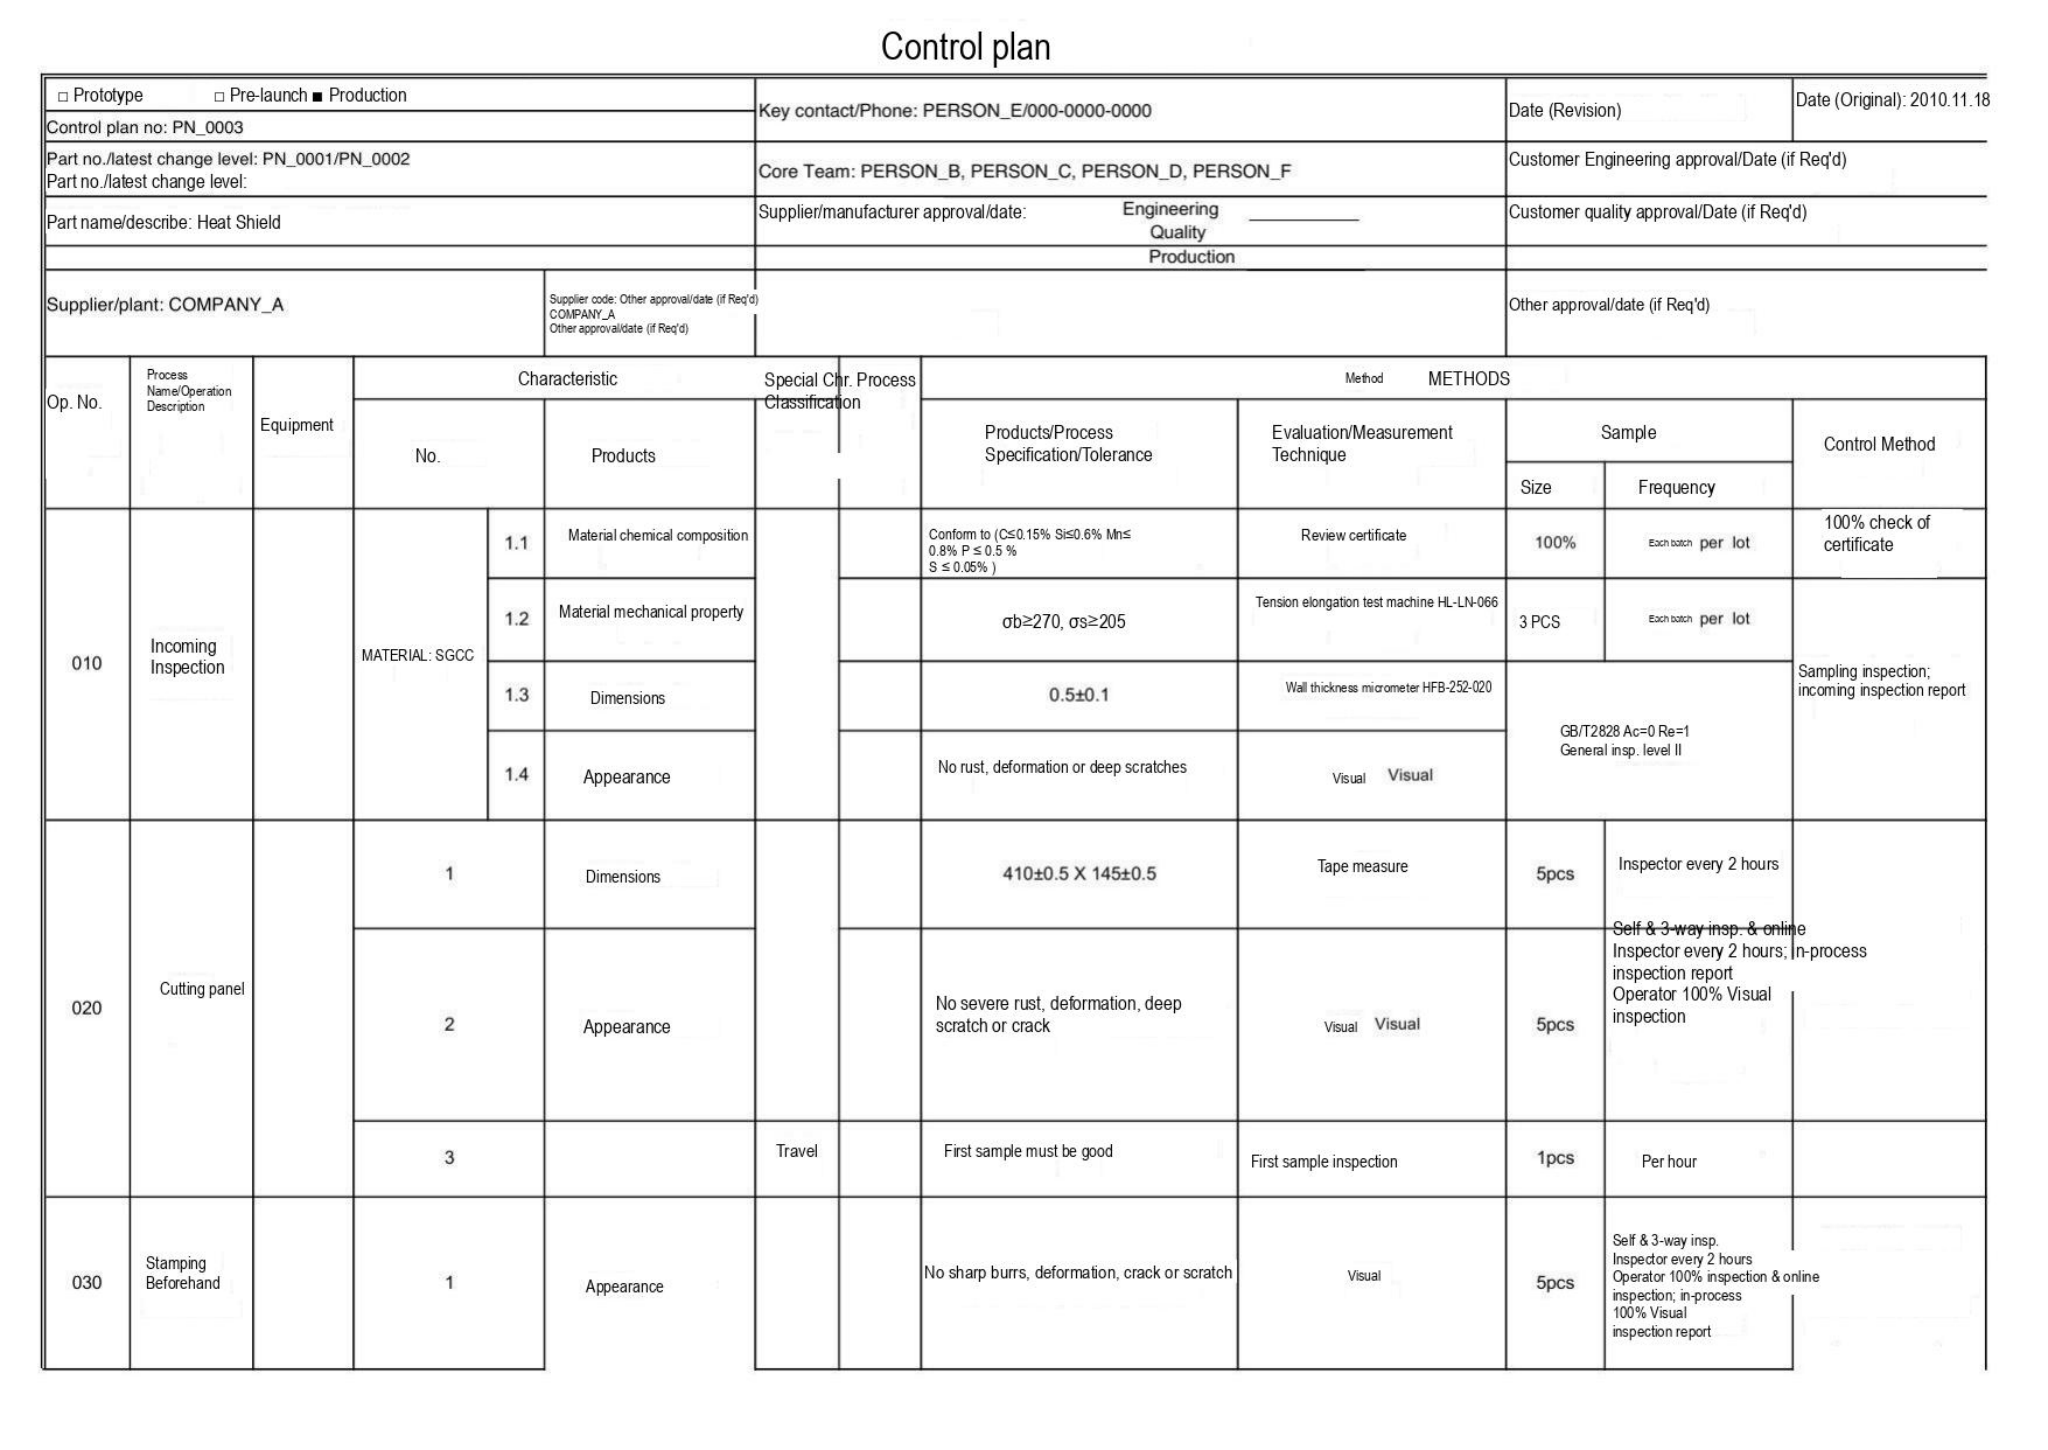# Control plan

| □ Prototype □ Pre-launch ■ Production | Key contact/Phone: PERSON_E/000-0000-0000 | Date (Revision) | Date (Original): 2010.11.18 |
|---|---|---|---|
| Control plan no: PN_0003 | | | |
| Part no./latest change level: PN_0001/PN_0002<br>Part no./latest change level: | Core Team: PERSON_B, PERSON_C, PERSON_D, PERSON_F | Customer Engineering approval/Date (if Req'd) | |
| Part name/describe: Heat Shield | Supplier/manufacturer approval/date: Engineering Quality Production | Customer quality approval/Date (if Req'd) | |
| Supplier/plant: COMPANY_A<br>Supplier code: Other approval/date (if Req'd) COMPANY_A Other approval/date (if Req'd) | | Other approval/date (if Req'd) | |

| Op. No. | Process Name/Operation Description | Equipment | Characteristic No. | | Characteristic Products | Special Chr. Process Classification | Method METHODS Products/Process Specification/Tolerance | Evaluation/Measurement Technique | Sample Size | Sample Frequency | Control Method |
|---|---|---|---|---|---|---|---|---|---|---|---|
| 010 | Incoming Inspection | | MATERIAL: SGCC | 1.1 | Material chemical composition | | Conform to (C≤0.15% Si≤0.6% Mn≤ 0.8% P ≤ 0.5 % S ≤ 0.05% ) | Review certificate | 100% | Each batch per lot | 100% check of certificate |
| | | | | 1.2 | Material mechanical property | | σb≥270, σs≥205 | Tension elongation test machine HL-LN-066 | 3 PCS | Each batch per lot | Sampling inspection; incoming inspection report |
| | | | | 1.3 | Dimensions | | 0.5±0.1 | Wall thickness micrometer HFB-252-020 | GB/T2828 Ac=0 Re=1 General insp. level II | | |
| | | | | 1.4 | Appearance | | No rust, deformation or deep scratches | Visual Visual | | | |
| 020 | Cutting panel | | 1 | | Dimensions | | 410±0.5 X 145±0.5 | Tape measure | 5pcs | Inspector every 2 hours | |
| | | | 2 | | Appearance | | No severe rust, deformation, deep scratch or crack | Visual Visual | 5pcs | Self & 3-way insp. & online Inspector every 2 hours; In-process inspection report Operator 100% Visual inspection | |
| | | | 3 | | | Travel | First sample must be good | First sample inspection | 1pcs | Per hour | |
| 030 | Stamping Beforehand | | 1 | | Appearance | | No sharp burrs, deformation, crack or scratch | Visual | 5pcs | Self & 3-way insp. Inspector every 2 hours Operator 100% inspection & online inspection; in-process 100% Visual inspection report | |
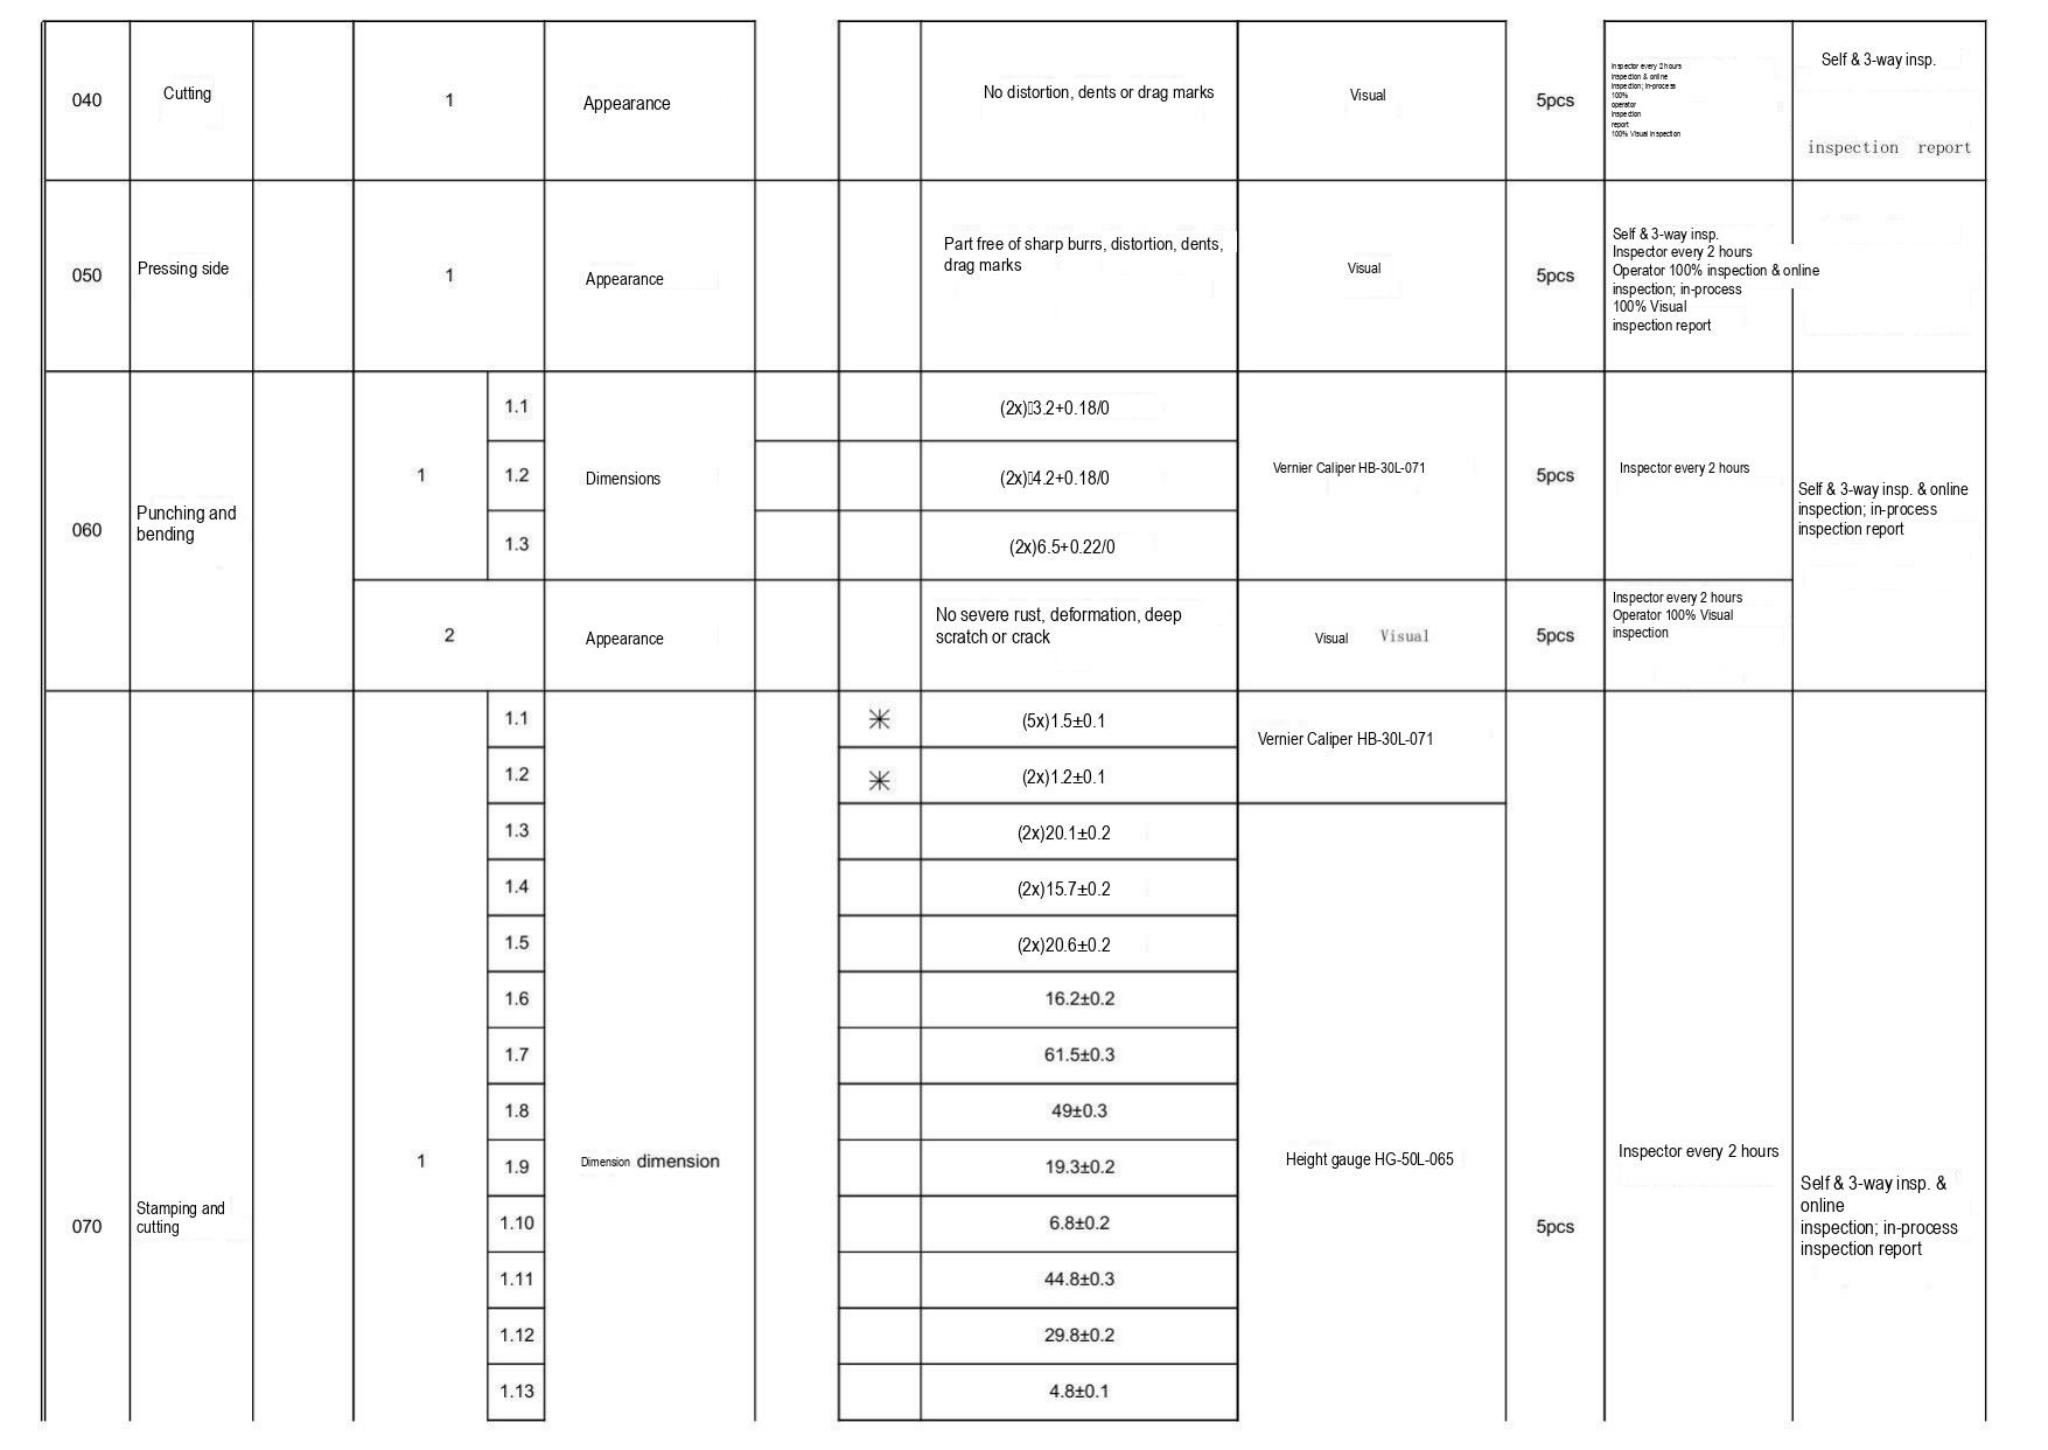| | | | | | | | | | | | | |
|---|---|---|---|---|---|---|---|---|---|---|---|---|
| 040 | Cutting | | 1 | | Appearance | | | No distortion, dents or drag marks | Visual | 5pcs | Inspector every 2 hours inspection & online inspection; in-process 100% operator inspection report 100% Visual inspection | Self & 3-way insp. inspection report |
| 050 | Pressing side | | 1 | | Appearance | | | Part free of sharp burrs, distortion, dents, drag marks | Visual | 5pcs | Self & 3-way insp. Inspector every 2 hours Operator 100% inspection & online inspection; in-process 100% Visual inspection report | |
| 060 | Punching and bending | | 1 | 1.1 | Dimensions | | | (2x)3.2+0.18/0 | Vernier Caliper HB-30L-071 | 5pcs | Inspector every 2 hours | Self & 3-way insp. & online inspection; in-process inspection report |
| | | | | 1.2 | | | | (2x)4.2+0.18/0 | | | | |
| | | | | 1.3 | | | | (2x)6.5+0.22/0 | | | | |
| | | | 2 | | Appearance | | | No severe rust, deformation, deep scratch or crack | Visual Visual | 5pcs | Inspector every 2 hours Operator 100% Visual inspection | |
| 070 | Stamping and cutting | | 1 | 1.1 | Dimension dimension | | ✳ | (5x)1.5±0.1 | Vernier Caliper HB-30L-071 | 5pcs | Inspector every 2 hours | Self & 3-way insp. & online inspection; in-process inspection report |
| | | | | 1.2 | | | ✳ | (2x)1.2±0.1 | | | | |
| | | | | 1.3 | | | | (2x)20.1±0.2 | Height gauge HG-50L-065 | | | |
| | | | | 1.4 | | | | (2x)15.7±0.2 | | | | |
| | | | | 1.5 | | | | (2x)20.6±0.2 | | | | |
| | | | | 1.6 | | | | 16.2±0.2 | | | | |
| | | | | 1.7 | | | | 61.5±0.3 | | | | |
| | | | | 1.8 | | | | 49±0.3 | | | | |
| | | | | 1.9 | | | | 19.3±0.2 | | | | |
| | | | | 1.10 | | | | 6.8±0.2 | | | | |
| | | | | 1.11 | | | | 44.8±0.3 | | | | |
| | | | | 1.12 | | | | 29.8±0.2 | | | | |
| | | | | 1.13 | | | | 4.8±0.1 | | | | |
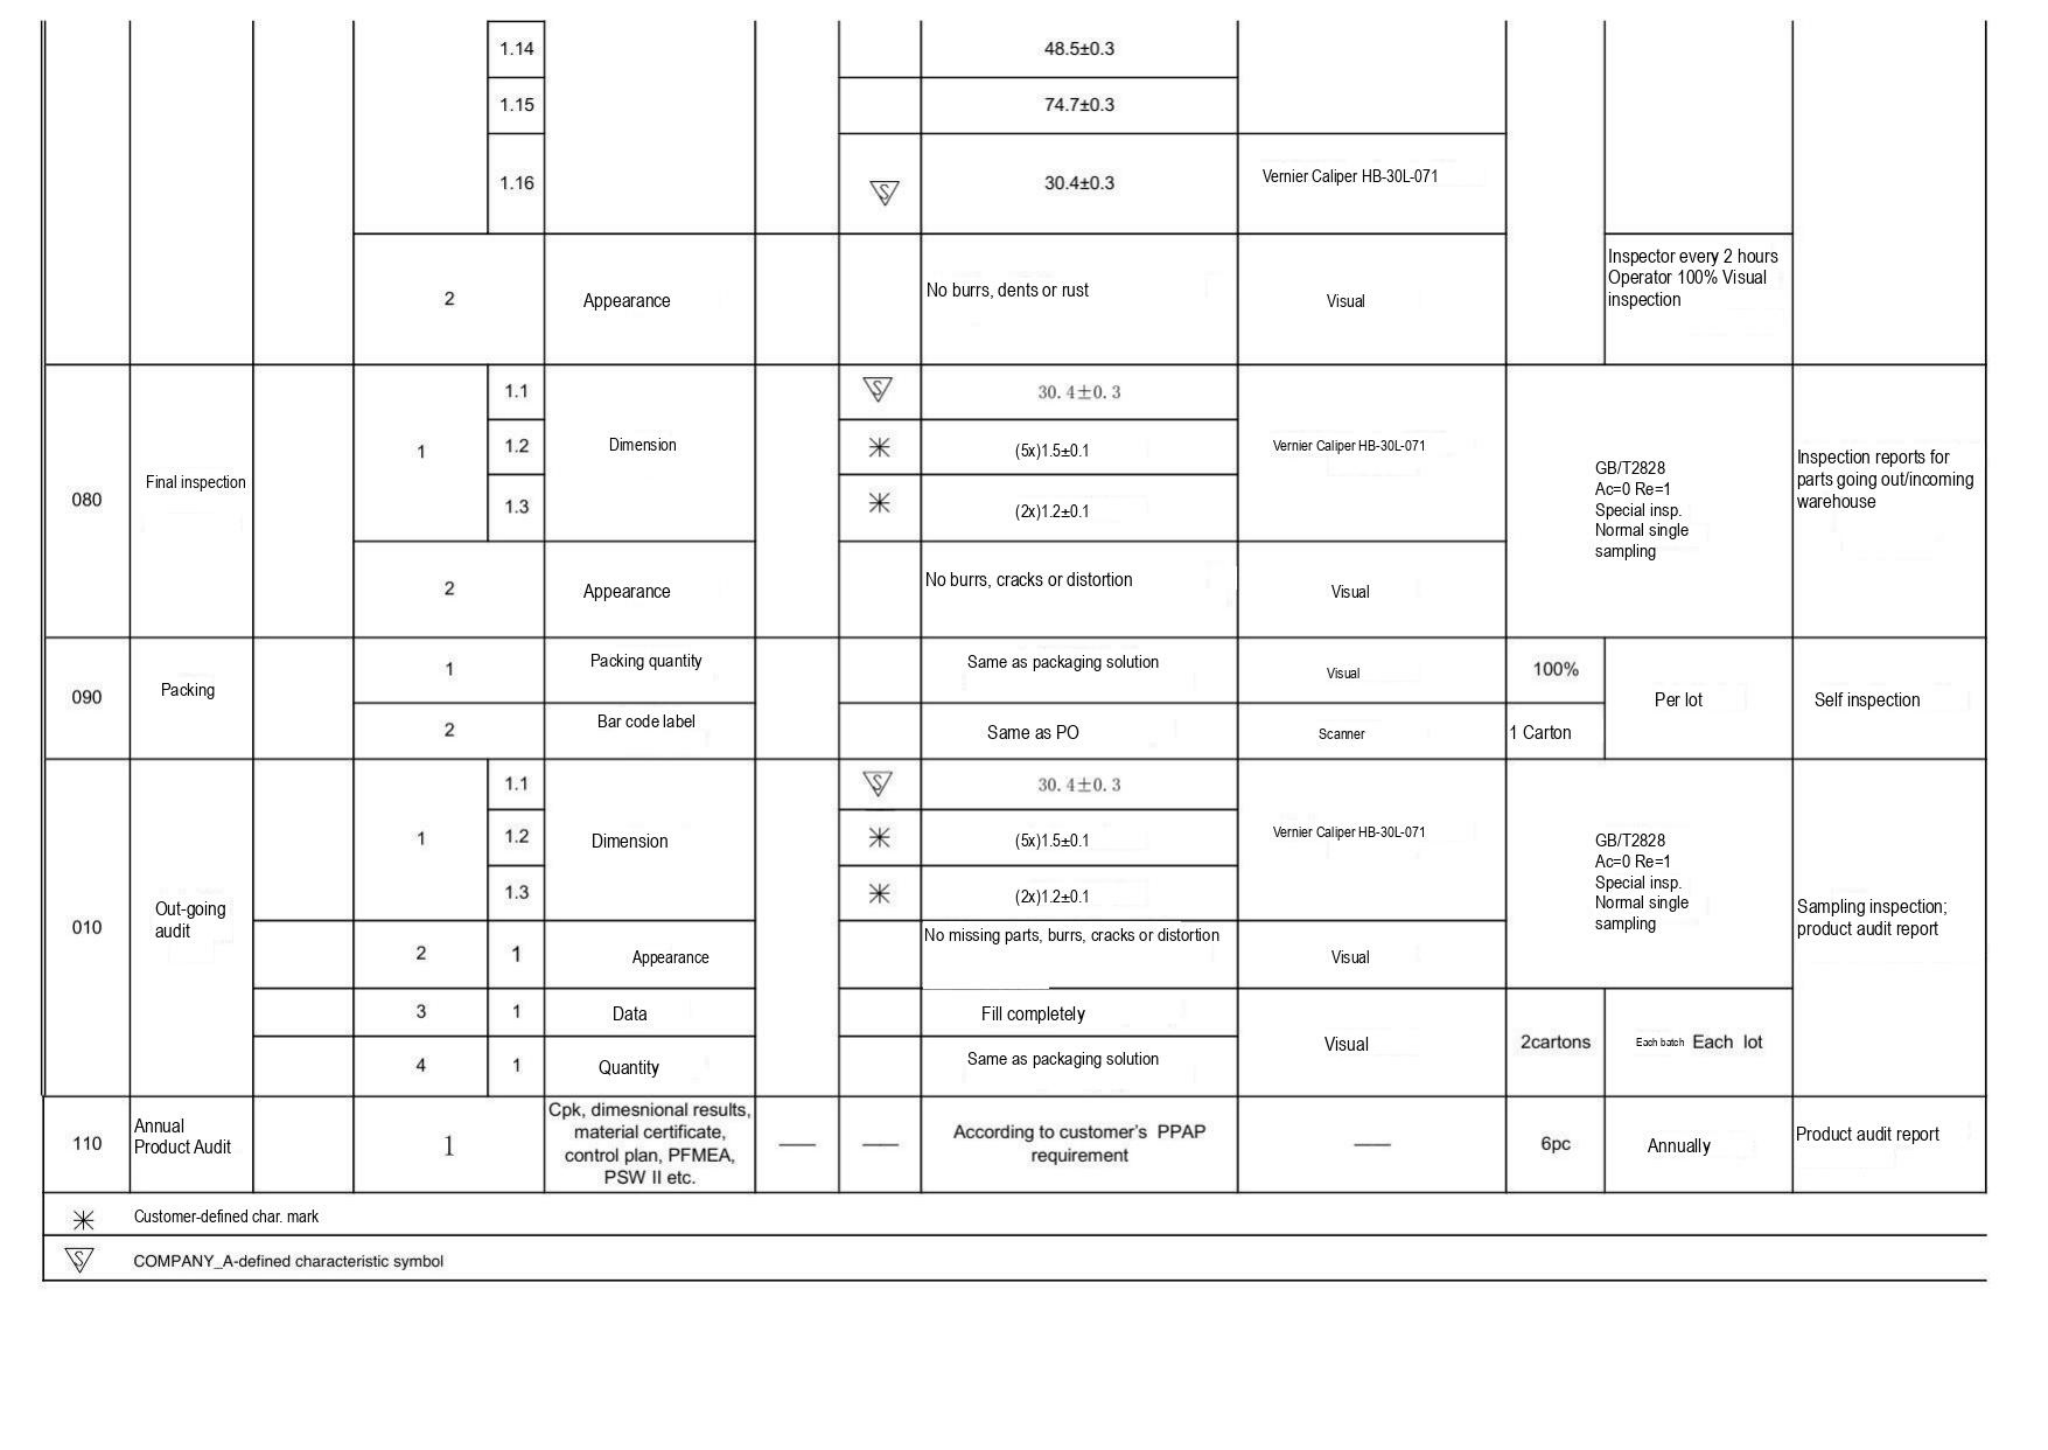|  |  |  |  |  |  |  |  |  |  |  |  |  |
|---|---|---|---|---|---|---|---|---|---|---|---|---|
|  |  |  |  | 1.14 |  |  |  | 48.5±0.3 |  |  |  |  |
|  |  |  |  | 1.15 |  |  |  | 74.7±0.3 |  |  |  |  |
|  |  |  |  | 1.16 |  |  | ▽S | 30.4±0.3 | Vernier Caliper HB-30L-071 |  |  |  |
|  |  |  | 2 |  | Appearance |  |  | No burrs, dents or rust | Visual |  | Inspector every 2 hours Operator 100% Visual inspection |  |
| 080 | Final inspection |  | 1 | 1.1 | Dimension |  | ▽S | 30.4±0.3 | Vernier Caliper HB-30L-071 | GB/T2828 Ac=0 Re=1 Special insp. Normal single sampling |  | Inspection reports for parts going out/incoming warehouse |
|  |  |  |  | 1.2 |  |  | ✳ | (5x)1.5±0.1 |  |  |  |  |
|  |  |  |  | 1.3 |  |  | ✳ | (2x)1.2±0.1 |  |  |  |  |
|  |  |  | 2 |  | Appearance |  |  | No burrs, cracks or distortion | Visual |  |  |  |
| 090 | Packing |  | 1 |  | Packing quantity |  |  | Same as packaging solution | Visual | 100% | Per lot | Self inspection |
|  |  |  | 2 |  | Bar code label |  |  | Same as PO | Scanner | 1 Carton |  |  |
| 010 | Out-going audit |  | 1 | 1.1 | Dimension |  | ▽S | 30.4±0.3 | Vernier Caliper HB-30L-071 | GB/T2828 Ac=0 Re=1 Special insp. Normal single sampling |  | Sampling inspection; product audit report |
|  |  |  |  | 1.2 |  |  | ✳ | (5x)1.5±0.1 |  |  |  |  |
|  |  |  |  | 1.3 |  |  | ✳ | (2x)1.2±0.1 |  |  |  |  |
|  |  |  | 2 | 1 | Appearance |  |  | No missing parts, burrs, cracks or distortion | Visual |  |  |  |
|  |  |  | 3 | 1 | Data |  |  | Fill completely | Visual | 2cartons | Each batch Each lot |  |
|  |  |  | 4 | 1 | Quantity |  |  | Same as packaging solution |  |  |  |  |
| 110 | Annual Product Audit |  | 1 |  | Cpk, dimesnional results, material certificate, control plan, PFMEA, PSW II etc. | — | — | According to customer's PPAP requirement | — | 6pc | Annually | Product audit report |

| | |
|---|---|
| ✳ | Customer-defined char. mark |
| ▽S | COMPANY_A-defined characteristic symbol |